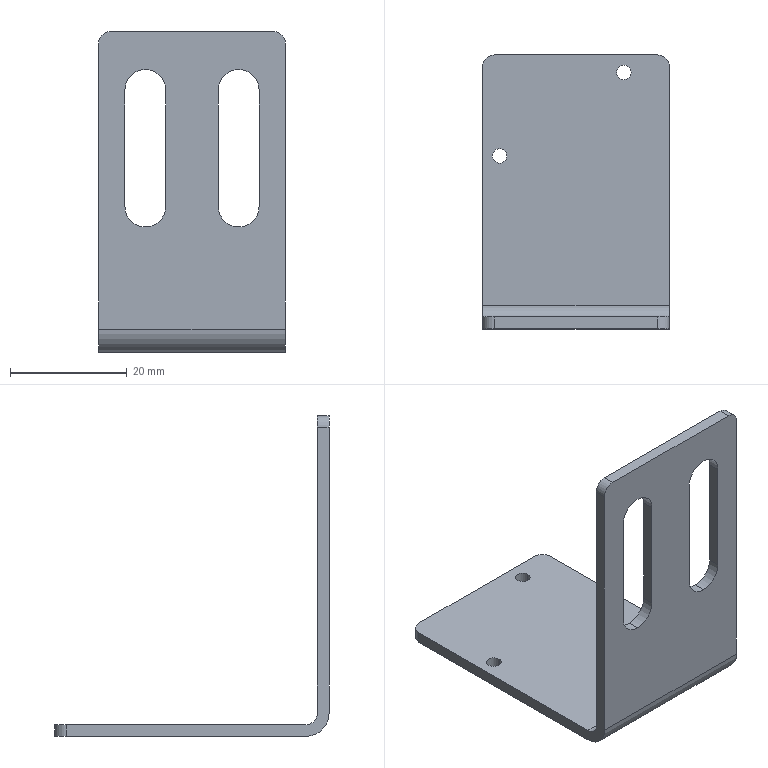Part | STEP file | 1 solid | 28 faces | box 32 x 47 x 55 mm | volume 5577 mm3 | cylinder 16 | plane 12 | commonest cylinder face diameters 7 x6 4 x5 2.5 x4 8 x1